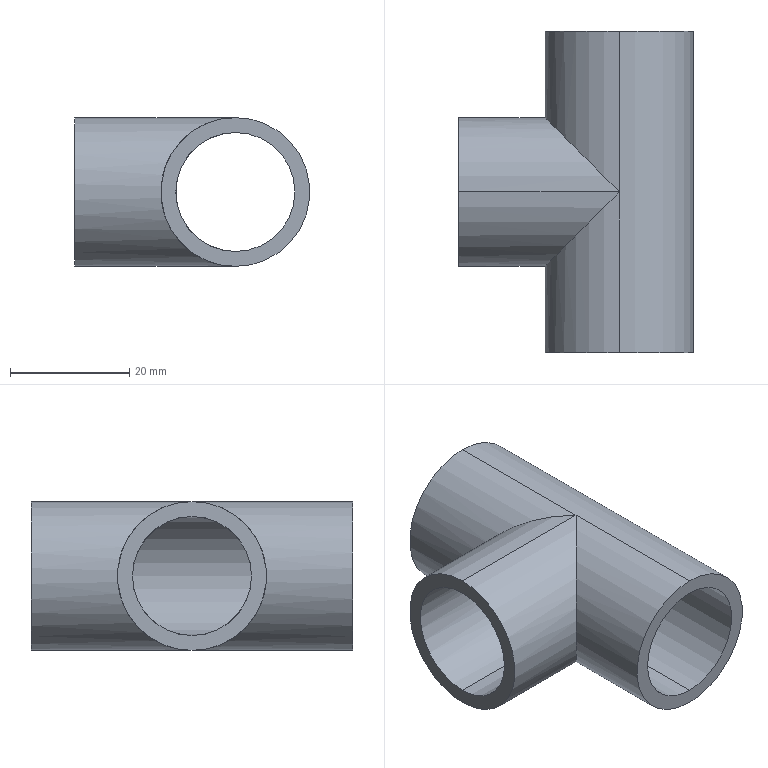Part | SolidWorks | features Cut 2, CirPattern 1, RefAxis 1, Revolution 1 | 1 solid | 13 faces | box 39.5 x 54 x 25 mm | volume 11772 mm3 | cylinder 10 | plane 3 | commonest cylinder face diameters 20 x5 25 x5
STEP:
#1=CARTESIAN_POINT('',(0.,27.,10.));
#2=VERTEX_POINT('',#1);
#3=CARTESIAN_POINT('',(0.,27.,-10.));
#4=VERTEX_POINT('',#3);
#5=CARTESIAN_POINT('',(0.,27.,0.));
#6=DIRECTION('',(0.,-1.,0.));
#7=DIRECTION('',(0.,0.,-1.));
#8=AXIS2_PLACEMENT_3D('',#5,#6,#7);
#9=CIRCLE('',#8,10.);
#10=EDGE_CURVE('',#2,#4,#9,.T.);
#11=ORIENTED_EDGE('',*,*,#10,.F.);
#12=CARTESIAN_POINT('',(0.,0.,10.));
#13=VERTEX_POINT('',#12);
#14=CARTESIAN_POINT('',(0.,0.,10.));
#15=DIRECTION('',(0.,-1.,0.));
#16=VECTOR('',#15,1000.);
#17=LINE('',#14,#16);
#18=EDGE_CURVE('',#2,#13,#17,.T.);
#19=ORIENTED_EDGE('',*,*,#18,.T.);
#20=CARTESIAN_POINT('',(0.,0.,-10.));
#21=VERTEX_POINT('',#20);
#22=CARTESIAN_POINT('',(0.,0.,10.));
#23=CARTESIAN_POINT('',(-20.,20.,10.));
#24=CARTESIAN_POINT('',(-20.,20.,-10.));
#25=CARTESIAN_POINT('',(0.,0.,-10.));
#26=(BOUNDED_CURVE()B_SPLINE_CURVE(3,(#22,#23,#24,#25),.UNSPECIFIED.,.F.,.F.)B_SPLINE_CURVE_WITH_KNOTS((4,4),(1.571,4.712),.UNSPECIFIED.)CURVE()GEOMETRIC_REPRESENTATION_ITEM()RATIONAL_B_SPLINE_CURVE((1.,0.3333,0.3333,1.))REPRESENTATION_ITEM(''));
#27=EDGE_CURVE('',#13,#21,#26,.T.);
#28=ORIENTED_EDGE('',*,*,#27,.T.);
#29=CARTESIAN_POINT('',(0.,0.,-10.));
#30=DIRECTION('',(0.,-1.,0.));
#31=VECTOR('',#30,1000.);
#32=LINE('',#29,#31);
#33=EDGE_CURVE('',#4,#21,#32,.T.);
#34=ORIENTED_EDGE('',*,*,#33,.F.);
#35=EDGE_LOOP('',(#11,#19,#28,#34));
#36=FACE_OUTER_BOUND('',#35,.T.);
#37=CARTESIAN_POINT('',(0.,0.,0.));
#38=DIRECTION('',(0.,-1.,0.));
#39=DIRECTION('',(0.,0.,-1.));
#40=AXIS2_PLACEMENT_3D('',#37,#38,#39);
#41=CYLINDRICAL_SURFACE('',#40,10.);
#42=ADVANCED_FACE('',(#36),#41,.F.);
#43=CARTESIAN_POINT('',(0.,0.,-10.));
#44=CARTESIAN_POINT('',(-20.,-20.,-10.));
#45=CARTESIAN_POINT('',(-20.,-20.,10.));
#46=CARTESIAN_POINT('',(0.,0.,10.));
#47=(BOUNDED_CURVE()B_SPLINE_CURVE(3,(#43,#44,#45,#46),.UNSPECIFIED.,.F.,.F.)B_SPLINE_CURVE_WITH_KNOTS((4,4),(4.712,7.854),.UNSPECIFIED.)CURVE()GEOMETRIC_REPRESENTATION_ITEM()RATIONAL_B_SPLINE_CURVE((1.,0.3333,0.3333,1.))REPRESENTATION_ITEM(''));
#48=EDGE_CURVE('',#21,#13,#47,.T.);
#49=ORIENTED_EDGE('',*,*,#48,.T.);
#50=CARTESIAN_POINT('',(0.,-27.,10.));
#51=VERTEX_POINT('',#50);
#52=CARTESIAN_POINT('',(0.,0.,10.));
#53=DIRECTION('',(0.,-1.,0.));
#54=VECTOR('',#53,1000.);
#55=LINE('',#52,#54);
#56=EDGE_CURVE('',#13,#51,#55,.T.);
#57=ORIENTED_EDGE('',*,*,#56,.T.);
#58=CARTESIAN_POINT('',(0.,-27.,-10.));
#59=VERTEX_POINT('',#58);
#60=CARTESIAN_POINT('',(0.,-27.,0.));
#61=DIRECTION('',(0.,1.,0.));
#62=DIRECTION('',(0.,0.,-1.));
#63=AXIS2_PLACEMENT_3D('',#60,#61,#62);
#64=CIRCLE('',#63,10.);
#65=EDGE_CURVE('',#59,#51,#64,.T.);
#66=ORIENTED_EDGE('',*,*,#65,.F.);
#67=CARTESIAN_POINT('',(0.,0.,-10.));
#68=DIRECTION('',(0.,-1.,0.));
#69=VECTOR('',#68,1000.);
#70=LINE('',#67,#69);
#71=EDGE_CURVE('',#21,#59,#70,.T.);
#72=ORIENTED_EDGE('',*,*,#71,.F.);
#73=EDGE_LOOP('',(#49,#57,#66,#72));
#74=FACE_OUTER_BOUND('',#73,.T.);
#75=CARTESIAN_POINT('',(0.,0.,0.));
#76=DIRECTION('',(0.,-1.,0.));
#77=DIRECTION('',(0.,0.,-1.));
#78=AXIS2_PLACEMENT_3D('',#75,#76,#77);
#79=CYLINDRICAL_SURFACE('',#78,10.);
#80=ADVANCED_FACE('',(#74),#79,.F.);
#81=CARTESIAN_POINT('',(0.,27.,-12.5));
#82=VERTEX_POINT('',#81);
#83=CARTESIAN_POINT('',(0.,27.,12.5));
#84=VERTEX_POINT('',#83);
#85=CARTESIAN_POINT('',(0.,27.,0.));
#86=DIRECTION('',(0.,-1.,0.));
#87=DIRECTION('',(0.,0.,-1.));
#88=AXIS2_PLACEMENT_3D('',#85,#86,#87);
#89=CIRCLE('',#88,12.5);
#90=EDGE_CURVE('',#82,#84,#89,.T.);
#91=ORIENTED_EDGE('',*,*,#90,.T.);
#92=CARTESIAN_POINT('',(0.,0.,12.5));
#93=VERTEX_POINT('',#92);
#94=CARTESIAN_POINT('',(0.,0.,12.5));
#95=DIRECTION('',(0.,-1.,0.));
#96=VECTOR('',#95,1000.);
#97=LINE('',#94,#96);
#98=EDGE_CURVE('',#84,#93,#97,.T.);
#99=ORIENTED_EDGE('',*,*,#98,.T.);
#100=CARTESIAN_POINT('',(0.,-27.,12.5));
#101=VERTEX_POINT('',#100);
#102=CARTESIAN_POINT('',(0.,0.,12.5));
#103=DIRECTION('',(0.,-1.,0.));
#104=VECTOR('',#103,1000.);
#105=LINE('',#102,#104);
#106=EDGE_CURVE('',#93,#101,#105,.T.);
#107=ORIENTED_EDGE('',*,*,#106,.T.);
#108=CARTESIAN_POINT('',(0.,-27.,-12.5));
#109=VERTEX_POINT('',#108);
#110=CARTESIAN_POINT('',(0.,-27.,0.));
#111=DIRECTION('',(0.,1.,0.));
#112=DIRECTION('',(0.,0.,-1.));
#113=AXIS2_PLACEMENT_3D('',#110,#111,#112);
#114=CIRCLE('',#113,12.5);
#115=EDGE_CURVE('',#101,#109,#114,.T.);
#116=ORIENTED_EDGE('',*,*,#115,.T.);
#117=CARTESIAN_POINT('',(0.,0.,-12.5));
#118=VERTEX_POINT('',#117);
#119=CARTESIAN_POINT('',(0.,0.,-12.5));
#120=DIRECTION('',(0.,-1.,0.));
#121=VECTOR('',#120,1000.);
#122=LINE('',#119,#121);
#123=EDGE_CURVE('',#118,#109,#122,.T.);
#124=ORIENTED_EDGE('',*,*,#123,.F.);
#125=CARTESIAN_POINT('',(0.,0.,-12.5));
#126=DIRECTION('',(0.,-1.,0.));
#127=VECTOR('',#126,1000.);
#128=LINE('',#125,#127);
#129=EDGE_CURVE('',#82,#118,#128,.T.);
#130=ORIENTED_EDGE('',*,*,#129,.F.);
#131=EDGE_LOOP('',(#91,#99,#107,#116,#124,#130));
#132=FACE_OUTER_BOUND('',#131,.T.);
#133=CARTESIAN_POINT('',(0.,0.,0.));
#134=DIRECTION('',(0.,-1.,0.));
#135=DIRECTION('',(0.,0.,-1.));
#136=AXIS2_PLACEMENT_3D('',#133,#134,#135);
#137=CYLINDRICAL_SURFACE('',#136,12.5);
#138=ADVANCED_FACE('',(#132),#137,.T.);
#139=ORIENTED_EDGE('',*,*,#98,.F.);
#140=CARTESIAN_POINT('',(0.,27.,0.));
#141=DIRECTION('',(0.,-1.,0.));
#142=DIRECTION('',(0.,0.,-1.));
#143=AXIS2_PLACEMENT_3D('',#140,#141,#142);
#144=CIRCLE('',#143,12.5);
#145=EDGE_CURVE('',#84,#82,#144,.T.);
#146=ORIENTED_EDGE('',*,*,#145,.T.);
#147=ORIENTED_EDGE('',*,*,#129,.T.);
#148=CARTESIAN_POINT('',(0.,0.,12.5));
#149=CARTESIAN_POINT('',(-25.,25.,12.5));
#150=CARTESIAN_POINT('',(-25.,25.,-12.5));
#151=CARTESIAN_POINT('',(0.,0.,-12.5));
#152=(BOUNDED_CURVE()B_SPLINE_CURVE(3,(#148,#149,#150,#151),.UNSPECIFIED.,.F.,.F.)B_SPLINE_CURVE_WITH_KNOTS((4,4),(1.571,4.712),.UNSPECIFIED.)CURVE()GEOMETRIC_REPRESENTATION_ITEM()RATIONAL_B_SPLINE_CURVE((1.,0.3333,0.3333,1.))REPRESENTATION_ITEM(''));
#153=EDGE_CURVE('',#93,#118,#152,.T.);
#154=ORIENTED_EDGE('',*,*,#153,.F.);
#155=EDGE_LOOP('',(#139,#146,#147,#154));
#156=FACE_OUTER_BOUND('',#155,.T.);
#157=CARTESIAN_POINT('',(0.,0.,0.));
#158=DIRECTION('',(0.,-1.,0.));
#159=DIRECTION('',(0.,0.,-1.));
#160=AXIS2_PLACEMENT_3D('',#157,#158,#159);
#161=CYLINDRICAL_SURFACE('',#160,12.5);
#162=ADVANCED_FACE('',(#156),#161,.T.);
#163=CARTESIAN_POINT('',(-27.,0.,10.));
#164=VERTEX_POINT('',#163);
#165=CARTESIAN_POINT('',(-27.,0.,-10.));
#166=VERTEX_POINT('',#165);
#167=CARTESIAN_POINT('',(-27.,0.,0.));
#168=DIRECTION('',(1.,0.,0.));
#169=DIRECTION('',(0.,0.,-1.));
#170=AXIS2_PLACEMENT_3D('',#167,#168,#169);
#171=CIRCLE('',#170,10.);
#172=EDGE_CURVE('',#164,#166,#171,.T.);
#173=ORIENTED_EDGE('',*,*,#172,.F.);
#174=CARTESIAN_POINT('',(0.,0.,10.));
#175=DIRECTION('',(1.,0.,0.));
#176=VECTOR('',#175,1000.);
#177=LINE('',#174,#176);
#178=EDGE_CURVE('',#164,#13,#177,.T.);
#179=ORIENTED_EDGE('',*,*,#178,.T.);
#180=ORIENTED_EDGE('',*,*,#48,.F.);
#181=CARTESIAN_POINT('',(0.,0.,-10.));
#182=DIRECTION('',(1.,0.,0.));
#183=VECTOR('',#182,1000.);
#184=LINE('',#181,#183);
#185=EDGE_CURVE('',#166,#21,#184,.T.);
#186=ORIENTED_EDGE('',*,*,#185,.F.);
#187=EDGE_LOOP('',(#173,#179,#180,#186));
#188=FACE_OUTER_BOUND('',#187,.T.);
#189=CARTESIAN_POINT('',(0.,0.,0.));
#190=DIRECTION('',(1.,0.,0.));
#191=DIRECTION('',(0.,0.,-1.));
#192=AXIS2_PLACEMENT_3D('',#189,#190,#191);
#193=CYLINDRICAL_SURFACE('',#192,10.);
#194=ADVANCED_FACE('',(#188),#193,.F.);
#195=CARTESIAN_POINT('',(-27.,0.,-12.5));
#196=VERTEX_POINT('',#195);
#197=CARTESIAN_POINT('',(-27.,0.,12.5));
#198=VERTEX_POINT('',#197);
#199=CARTESIAN_POINT('',(-27.,0.,0.));
#200=DIRECTION('',(1.,0.,0.));
#201=DIRECTION('',(0.,0.,-1.));
#202=AXIS2_PLACEMENT_3D('',#199,#200,#201);
#203=CIRCLE('',#202,12.5);
#204=EDGE_CURVE('',#196,#198,#203,.T.);
#205=ORIENTED_EDGE('',*,*,#204,.T.);
#206=CARTESIAN_POINT('',(0.,0.,12.5));
#207=DIRECTION('',(1.,0.,0.));
#208=VECTOR('',#207,1000.);
#209=LINE('',#206,#208);
#210=EDGE_CURVE('',#198,#93,#209,.T.);
#211=ORIENTED_EDGE('',*,*,#210,.T.);
#212=ORIENTED_EDGE('',*,*,#153,.T.);
#213=CARTESIAN_POINT('',(0.,0.,-12.5));
#214=DIRECTION('',(1.,0.,0.));
#215=VECTOR('',#214,1000.);
#216=LINE('',#213,#215);
#217=EDGE_CURVE('',#196,#118,#216,.T.);
#218=ORIENTED_EDGE('',*,*,#217,.F.);
#219=EDGE_LOOP('',(#205,#211,#212,#218));
#220=FACE_OUTER_BOUND('',#219,.T.);
#221=CARTESIAN_POINT('',(0.,0.,0.));
#222=DIRECTION('',(1.,0.,0.));
#223=DIRECTION('',(0.,0.,-1.));
#224=AXIS2_PLACEMENT_3D('',#221,#222,#223);
#225=CYLINDRICAL_SURFACE('',#224,12.5);
#226=ADVANCED_FACE('',(#220),#225,.T.);
#227=ORIENTED_EDGE('',*,*,#210,.F.);
#228=CARTESIAN_POINT('',(-27.,0.,0.));
#229=DIRECTION('',(1.,0.,0.));
#230=DIRECTION('',(0.,0.,-1.));
#231=AXIS2_PLACEMENT_3D('',#228,#229,#230);
#232=CIRCLE('',#231,12.5);
#233=EDGE_CURVE('',#198,#196,#232,.T.);
#234=ORIENTED_EDGE('',*,*,#233,.T.);
#235=ORIENTED_EDGE('',*,*,#217,.T.);
#236=CARTESIAN_POINT('',(0.,0.,12.5));
#237=CARTESIAN_POINT('',(-25.,-25.,12.5));
#238=CARTESIAN_POINT('',(-25.,-25.,-12.5));
#239=CARTESIAN_POINT('',(0.,0.,-12.5));
#240=(BOUNDED_CURVE()B_SPLINE_CURVE(3,(#236,#237,#238,#239),.UNSPECIFIED.,.F.,.F.)B_SPLINE_CURVE_WITH_KNOTS((4,4),(1.571,4.712),.UNSPECIFIED.)CURVE()GEOMETRIC_REPRESENTATION_ITEM()RATIONAL_B_SPLINE_CURVE((1.,0.3333,0.3333,1.))REPRESENTATION_ITEM(''));
#241=EDGE_CURVE('',#93,#118,#240,.T.);
#242=ORIENTED_EDGE('',*,*,#241,.F.);
#243=EDGE_LOOP('',(#227,#234,#235,#242));
#244=FACE_OUTER_BOUND('',#243,.T.);
#245=CARTESIAN_POINT('',(0.,0.,0.));
#246=DIRECTION('',(1.,0.,0.));
#247=DIRECTION('',(0.,0.,-1.));
#248=AXIS2_PLACEMENT_3D('',#245,#246,#247);
#249=CYLINDRICAL_SURFACE('',#248,12.5);
#250=ADVANCED_FACE('',(#244),#249,.T.);
#251=ORIENTED_EDGE('',*,*,#178,.F.);
#252=CARTESIAN_POINT('',(-27.,0.,0.));
#253=DIRECTION('',(1.,0.,0.));
#254=DIRECTION('',(0.,0.,-1.));
#255=AXIS2_PLACEMENT_3D('',#252,#253,#254);
#256=CIRCLE('',#255,10.);
#257=EDGE_CURVE('',#166,#164,#256,.T.);
#258=ORIENTED_EDGE('',*,*,#257,.F.);
#259=ORIENTED_EDGE('',*,*,#185,.T.);
#260=ORIENTED_EDGE('',*,*,#27,.F.);
#261=EDGE_LOOP('',(#251,#258,#259,#260));
#262=FACE_OUTER_BOUND('',#261,.T.);
#263=CARTESIAN_POINT('',(0.,0.,0.));
#264=DIRECTION('',(1.,0.,0.));
#265=DIRECTION('',(0.,0.,-1.));
#266=AXIS2_PLACEMENT_3D('',#263,#264,#265);
#267=CYLINDRICAL_SURFACE('',#266,10.);
#268=ADVANCED_FACE('',(#262),#267,.F.);
#269=ORIENTED_EDGE('',*,*,#204,.F.);
#270=ORIENTED_EDGE('',*,*,#233,.F.);
#271=EDGE_LOOP('',(#269,#270));
#272=FACE_OUTER_BOUND('',#271,.T.);
#273=ORIENTED_EDGE('',*,*,#257,.T.);
#274=ORIENTED_EDGE('',*,*,#172,.T.);
#275=EDGE_LOOP('',(#273,#274));
#276=FACE_BOUND('',#275,.T.);
#277=CARTESIAN_POINT('',(-27.,-10.,0.));
#278=DIRECTION('',(1.,0.,0.));
#279=DIRECTION('',(0.,0.,-1.));
#280=AXIS2_PLACEMENT_3D('',#277,#278,#279);
#281=PLANE('',#280);
#282=ADVANCED_FACE('',(#272,#276),#281,.F.);
#283=CARTESIAN_POINT('',(0.,-27.,0.));
#284=DIRECTION('',(0.,1.,0.));
#285=DIRECTION('',(0.,0.,-1.));
#286=AXIS2_PLACEMENT_3D('',#283,#284,#285);
#287=CIRCLE('',#286,12.5);
#288=EDGE_CURVE('',#109,#101,#287,.T.);
#289=ORIENTED_EDGE('',*,*,#288,.F.);
#290=ORIENTED_EDGE('',*,*,#115,.F.);
#291=EDGE_LOOP('',(#289,#290));
#292=FACE_OUTER_BOUND('',#291,.T.);
#293=ORIENTED_EDGE('',*,*,#65,.T.);
#294=CARTESIAN_POINT('',(0.,-27.,0.));
#295=DIRECTION('',(0.,1.,0.));
#296=DIRECTION('',(0.,0.,-1.));
#297=AXIS2_PLACEMENT_3D('',#294,#295,#296);
#298=CIRCLE('',#297,10.);
#299=EDGE_CURVE('',#51,#59,#298,.T.);
#300=ORIENTED_EDGE('',*,*,#299,.T.);
#301=EDGE_LOOP('',(#293,#300));
#302=FACE_BOUND('',#301,.T.);
#303=CARTESIAN_POINT('',(10.,-27.,0.));
#304=DIRECTION('',(0.,1.,0.));
#305=DIRECTION('',(0.,0.,-1.));
#306=AXIS2_PLACEMENT_3D('',#303,#304,#305);
#307=PLANE('',#306);
#308=ADVANCED_FACE('',(#292,#302),#307,.F.);
#309=ORIENTED_EDGE('',*,*,#106,.F.);
#310=ORIENTED_EDGE('',*,*,#241,.T.);
#311=ORIENTED_EDGE('',*,*,#123,.T.);
#312=ORIENTED_EDGE('',*,*,#288,.T.);
#313=EDGE_LOOP('',(#309,#310,#311,#312));
#314=FACE_OUTER_BOUND('',#313,.T.);
#315=CARTESIAN_POINT('',(0.,0.,0.));
#316=DIRECTION('',(0.,-1.,0.));
#317=DIRECTION('',(0.,0.,-1.));
#318=AXIS2_PLACEMENT_3D('',#315,#316,#317);
#319=CYLINDRICAL_SURFACE('',#318,12.5);
#320=ADVANCED_FACE('',(#314),#319,.T.);
#321=ORIENTED_EDGE('',*,*,#90,.F.);
#322=ORIENTED_EDGE('',*,*,#145,.F.);
#323=EDGE_LOOP('',(#321,#322));
#324=FACE_OUTER_BOUND('',#323,.T.);
#325=CARTESIAN_POINT('',(0.,27.,0.));
#326=DIRECTION('',(0.,-1.,0.));
#327=DIRECTION('',(0.,0.,-1.));
#328=AXIS2_PLACEMENT_3D('',#325,#326,#327);
#329=CIRCLE('',#328,10.);
#330=EDGE_CURVE('',#4,#2,#329,.T.);
#331=ORIENTED_EDGE('',*,*,#330,.T.);
#332=ORIENTED_EDGE('',*,*,#10,.T.);
#333=EDGE_LOOP('',(#331,#332));
#334=FACE_BOUND('',#333,.T.);
#335=CARTESIAN_POINT('',(-10.,27.,0.));
#336=DIRECTION('',(0.,-1.,0.));
#337=DIRECTION('',(0.,0.,-1.));
#338=AXIS2_PLACEMENT_3D('',#335,#336,#337);
#339=PLANE('',#338);
#340=ADVANCED_FACE('',(#324,#334),#339,.F.);
#341=ORIENTED_EDGE('',*,*,#18,.F.);
#342=ORIENTED_EDGE('',*,*,#330,.F.);
#343=ORIENTED_EDGE('',*,*,#33,.T.);
#344=ORIENTED_EDGE('',*,*,#71,.T.);
#345=ORIENTED_EDGE('',*,*,#299,.F.);
#346=ORIENTED_EDGE('',*,*,#56,.F.);
#347=EDGE_LOOP('',(#341,#342,#343,#344,#345,#346));
#348=FACE_OUTER_BOUND('',#347,.T.);
#349=CARTESIAN_POINT('',(0.,0.,0.));
#350=DIRECTION('',(0.,-1.,0.));
#351=DIRECTION('',(0.,0.,-1.));
#352=AXIS2_PLACEMENT_3D('',#349,#350,#351);
#353=CYLINDRICAL_SURFACE('',#352,10.);
#354=ADVANCED_FACE('',(#348),#353,.F.);
#355=CLOSED_SHELL('',(#42,#80,#138,#162,#194,#226,#250,#268,#282,#308,#320,#340,#354));
#356=MANIFOLD_SOLID_BREP('',#355);
#357=CARTESIAN_POINT('',(0.,0.,0.));
#358=DIRECTION('',(0.,0.,1.));
#359=DIRECTION('',(1.,0.,0.));
#360=AXIS2_PLACEMENT_3D('',#357,#358,#359);
#361=(LENGTH_UNIT()NAMED_UNIT(*)SI_UNIT(.MILLI.,.METRE.));
#362=UNCERTAINTY_MEASURE_WITH_UNIT(LENGTH_MEASURE(0.00001),#361,'','');
#363=(NAMED_UNIT(*)PLANE_ANGLE_UNIT()SI_UNIT($,.RADIAN.));
#364=(NAMED_UNIT(*)SI_UNIT($,.STERADIAN.)SOLID_ANGLE_UNIT());
#365=(GEOMETRIC_REPRESENTATION_CONTEXT(3)GLOBAL_UNCERTAINTY_ASSIGNED_CONTEXT((#362))GLOBAL_UNIT_ASSIGNED_CONTEXT((#361,#363,#364))REPRESENTATION_CONTEXT('',''));
#366=ADVANCED_BREP_SHAPE_REPRESENTATION('',(#356,#360),#365);